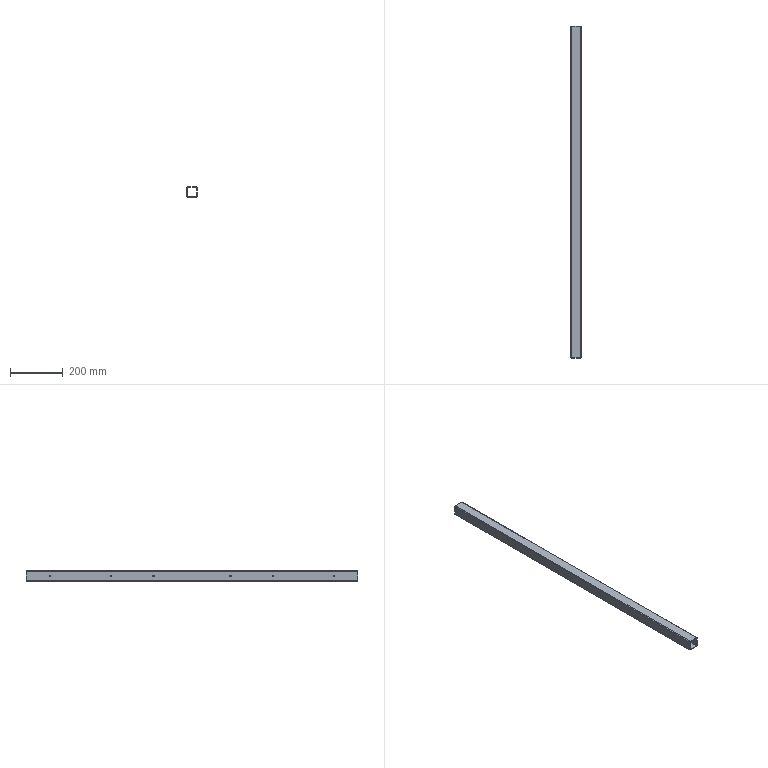Part | NX | features BREP 1 | 1 solid | 50 faces | box 40 x 1258 x 40 mm | volume 371774 mm3 | cylinder 40 | plane 10 | commonest cylinder face diameters 6.5 x12 2 x8 7 x8 15 x8 6 x4